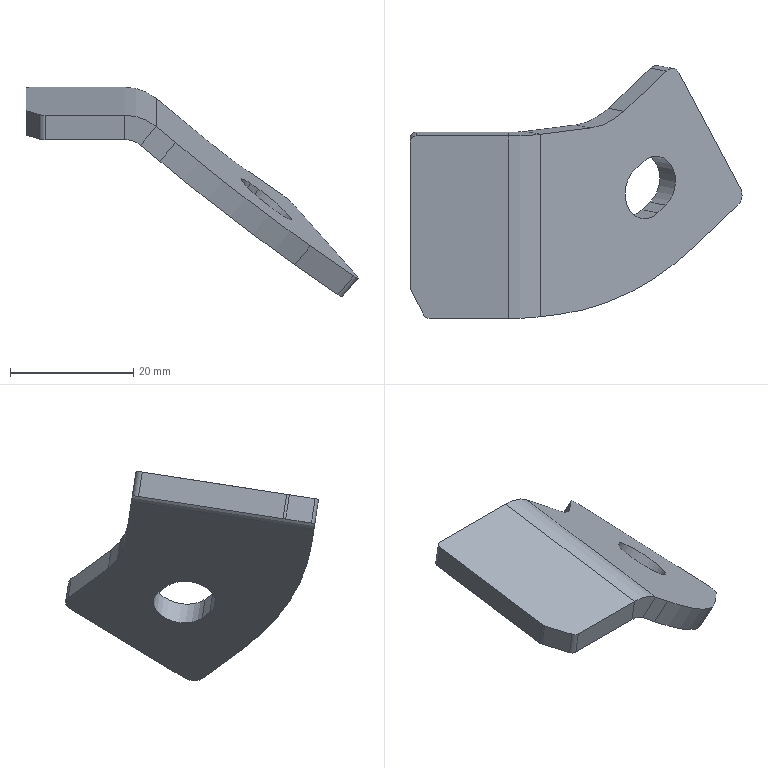Part | SolidWorks | features BaseBody 1 | 1 solid | 28 faces | box 53.982 x 41.139 x 34.078 mm | volume 6539 mm3 | plane 16 | cylinder 11 | spline 1 | commonest cylinder face diameters 2 x3 4 x2 9 x2 8 x1 16 x1 26 x1
STEP:
#1=CARTESIAN_POINT('',(-301.692,285.702,-816.532));
#2=VERTEX_POINT('',#1);
#3=CARTESIAN_POINT('',(-299.57,281.523,-817.174));
#4=VERTEX_POINT('',#3);
#5=CARTESIAN_POINT('',(-301.692,285.702,-816.532));
#6=CARTESIAN_POINT('',(-301.439,285.211,-816.607));
#7=CARTESIAN_POINT('',(-300.904,284.166,-816.768));
#8=CARTESIAN_POINT('',(-300.195,282.773,-816.982));
#9=CARTESIAN_POINT('',(-299.746,281.876,-817.12));
#10=CARTESIAN_POINT('',(-299.57,281.523,-817.174));
#11=B_SPLINE_CURVE_WITH_KNOTS('',3,(#5,#6,#7,#8,#9,#10),.UNSPECIFIED.,.F.,.F.,(4,1,1,4),(0.,0.3455,0.7405,1.),.UNSPECIFIED.);
#12=EDGE_CURVE('',#2,#4,#11,.T.);
#13=ORIENTED_EDGE('',*,*,#12,.F.);
#14=CARTESIAN_POINT('',(-301.8,286.15,-816.463));
#15=VERTEX_POINT('',#14);
#16=CARTESIAN_POINT('',(-300.8,286.15,-816.463));
#17=DIRECTION('',(0.,-0.1519,0.9884));
#18=DIRECTION('',(-1.,0.,0.));
#19=AXIS2_PLACEMENT_3D('',#16,#17,#18);
#20=CIRCLE('',#19,1.);
#21=EDGE_CURVE('',#15,#2,#20,.T.);
#22=ORIENTED_EDGE('',*,*,#21,.F.);
#23=CARTESIAN_POINT('',(-301.8,309.634,-812.853));
#24=VERTEX_POINT('',#23);
#25=CARTESIAN_POINT('',(-301.8,286.15,-816.463));
#26=DIRECTION('',(0.,0.9884,0.1519));
#27=VECTOR('',#26,1000.);
#28=LINE('',#25,#27);
#29=EDGE_CURVE('',#15,#24,#28,.T.);
#30=ORIENTED_EDGE('',*,*,#29,.T.);
#31=CARTESIAN_POINT('',(-300.8,310.623,-812.701));
#32=VERTEX_POINT('',#31);
#33=CARTESIAN_POINT('',(-300.8,309.634,-812.853));
#34=DIRECTION('',(0.,-0.1519,0.9884));
#35=DIRECTION('',(0.,0.9884,0.1519));
#36=AXIS2_PLACEMENT_3D('',#33,#34,#35);
#37=CIRCLE('',#36,1.);
#38=EDGE_CURVE('',#32,#24,#37,.T.);
#39=ORIENTED_EDGE('',*,*,#38,.F.);
#40=CARTESIAN_POINT('',(-285.757,310.623,-812.701));
#41=VERTEX_POINT('',#40);
#42=CARTESIAN_POINT('',(-300.8,310.623,-812.701));
#43=DIRECTION('',(1.,0.,0.));
#44=VECTOR('',#43,1000.);
#45=LINE('',#42,#44);
#46=EDGE_CURVE('',#32,#41,#45,.T.);
#47=ORIENTED_EDGE('',*,*,#46,.T.);
#48=CARTESIAN_POINT('',(-285.757,280.971,-817.259));
#49=VERTEX_POINT('',#48);
#50=CARTESIAN_POINT('',(-285.757,310.623,-812.701));
#51=DIRECTION('',(0.,-0.9884,-0.1519));
#52=VECTOR('',#51,1000.);
#53=LINE('',#50,#52);
#54=EDGE_CURVE('',#41,#49,#53,.T.);
#55=ORIENTED_EDGE('',*,*,#54,.T.);
#56=CARTESIAN_POINT('',(-298.673,280.971,-817.259));
#57=VERTEX_POINT('',#56);
#58=CARTESIAN_POINT('',(-285.757,280.971,-817.259));
#59=DIRECTION('',(-1.,0.,0.));
#60=VECTOR('',#59,1000.);
#61=LINE('',#58,#60);
#62=EDGE_CURVE('',#49,#57,#61,.T.);
#63=ORIENTED_EDGE('',*,*,#62,.T.);
#64=CARTESIAN_POINT('',(-298.673,281.959,-817.107));
#65=DIRECTION('',(0.,-0.1519,0.9884));
#66=DIRECTION('',(-0.8972,-0.4365,-0.0671));
#67=AXIS2_PLACEMENT_3D('',#64,#65,#66);
#68=CIRCLE('',#67,1.);
#69=EDGE_CURVE('',#4,#57,#68,.T.);
#70=ORIENTED_EDGE('',*,*,#69,.F.);
#71=EDGE_LOOP('',(#13,#22,#30,#39,#47,#55,#63,#70));
#72=FACE_OUTER_BOUND('',#71,.T.);
#73=CARTESIAN_POINT('',(-79.9,310.623,-812.701));
#74=DIRECTION('',(0.,-0.1519,0.9884));
#75=DIRECTION('',(-1.,0.,0.));
#76=AXIS2_PLACEMENT_3D('',#73,#74,#75);
#77=PLANE('',#76);
#78=ADVANCED_FACE('',(#72),#77,.F.);
#79=CARTESIAN_POINT('',(-298.673,280.363,-813.306));
#80=VERTEX_POINT('',#79);
#81=CARTESIAN_POINT('',(-298.673,280.363,-813.306));
#82=DIRECTION('',(0.,0.1519,-0.9884));
#83=VECTOR('',#82,1000.);
#84=LINE('',#81,#83);
#85=EDGE_CURVE('',#80,#57,#84,.T.);
#86=ORIENTED_EDGE('',*,*,#85,.F.);
#87=CARTESIAN_POINT('',(-299.57,280.915,-813.221));
#88=VERTEX_POINT('',#87);
#89=CARTESIAN_POINT('',(-298.673,281.352,-813.154));
#90=DIRECTION('',(0.,0.1519,-0.9884));
#91=DIRECTION('',(0.,-0.9884,-0.1519));
#92=AXIS2_PLACEMENT_3D('',#89,#90,#91);
#93=CIRCLE('',#92,1.);
#94=EDGE_CURVE('',#80,#88,#93,.T.);
#95=ORIENTED_EDGE('',*,*,#94,.T.);
#96=CARTESIAN_POINT('',(-299.57,281.523,-817.174));
#97=DIRECTION('',(0.,-0.1519,0.9884));
#98=VECTOR('',#97,1000.);
#99=LINE('',#96,#98);
#100=EDGE_CURVE('',#4,#88,#99,.T.);
#101=ORIENTED_EDGE('',*,*,#100,.F.);
#102=ORIENTED_EDGE('',*,*,#69,.T.);
#103=EDGE_LOOP('',(#86,#95,#101,#102));
#104=FACE_OUTER_BOUND('',#103,.T.);
#105=CARTESIAN_POINT('',(-298.673,281.656,-815.131));
#106=DIRECTION('',(0.,0.1519,-0.9884));
#107=DIRECTION('',(0.,-0.9884,-0.1519));
#108=AXIS2_PLACEMENT_3D('',#105,#106,#107);
#109=CYLINDRICAL_SURFACE('',#108,1.);
#110=ADVANCED_FACE('',(#104),#109,.T.);
#111=CARTESIAN_POINT('',(-301.692,285.094,-812.578));
#112=VERTEX_POINT('',#111);
#113=CARTESIAN_POINT('',(-299.57,280.915,-813.221));
#114=CARTESIAN_POINT('',(-299.746,281.269,-813.166));
#115=CARTESIAN_POINT('',(-300.195,282.166,-813.029));
#116=CARTESIAN_POINT('',(-300.904,283.558,-812.815));
#117=CARTESIAN_POINT('',(-301.439,284.603,-812.654));
#118=CARTESIAN_POINT('',(-301.692,285.094,-812.578));
#119=B_SPLINE_CURVE_WITH_KNOTS('',3,(#113,#114,#115,#116,#117,#118),.UNSPECIFIED.,.F.,.F.,(4,1,1,4),(0.,0.2595,0.6545,1.),.UNSPECIFIED.);
#120=EDGE_CURVE('',#88,#112,#119,.T.);
#121=ORIENTED_EDGE('',*,*,#120,.T.);
#122=CARTESIAN_POINT('',(-301.692,285.094,-812.578));
#123=DIRECTION('',(0.,0.1519,-0.9884));
#124=VECTOR('',#123,1000.);
#125=LINE('',#122,#124);
#126=EDGE_CURVE('',#112,#2,#125,.T.);
#127=ORIENTED_EDGE('',*,*,#126,.T.);
#128=ORIENTED_EDGE('',*,*,#12,.T.);
#129=ORIENTED_EDGE('',*,*,#100,.T.);
#130=EDGE_LOOP('',(#121,#127,#128,#129));
#131=FACE_OUTER_BOUND('',#130,.T.);
#132=CARTESIAN_POINT('',(-301.692,285.702,-816.532));
#133=CARTESIAN_POINT('',(-301.692,285.094,-812.578));
#134=CARTESIAN_POINT('',(-301.439,285.211,-816.607));
#135=CARTESIAN_POINT('',(-301.439,284.603,-812.654));
#136=CARTESIAN_POINT('',(-300.904,284.166,-816.768));
#137=CARTESIAN_POINT('',(-300.904,283.558,-812.815));
#138=CARTESIAN_POINT('',(-300.195,282.773,-816.982));
#139=CARTESIAN_POINT('',(-300.195,282.166,-813.029));
#140=CARTESIAN_POINT('',(-299.746,281.876,-817.12));
#141=CARTESIAN_POINT('',(-299.746,281.269,-813.166));
#142=CARTESIAN_POINT('',(-299.57,281.523,-817.174));
#143=CARTESIAN_POINT('',(-299.57,280.915,-813.221));
#144=B_SPLINE_SURFACE_WITH_KNOTS('',3,1,((#132,#133),(#134,#135),(#136,#137),(#138,#139),(#140,#141),(#142,#143)),.UNSPECIFIED.,.F.,.F.,.F.,(4,1,1,4),(2,2),(0.0124,0.3492,0.7341,0.987),(0.,1.),.UNSPECIFIED.);
#145=ADVANCED_FACE('',(#131),#144,.T.);
#146=CARTESIAN_POINT('',(-301.8,285.542,-812.51));
#147=VERTEX_POINT('',#146);
#148=CARTESIAN_POINT('',(-301.8,286.15,-816.463));
#149=DIRECTION('',(0.,-0.1519,0.9884));
#150=VECTOR('',#149,1000.);
#151=LINE('',#148,#150);
#152=EDGE_CURVE('',#15,#147,#151,.T.);
#153=ORIENTED_EDGE('',*,*,#152,.F.);
#154=ORIENTED_EDGE('',*,*,#21,.T.);
#155=ORIENTED_EDGE('',*,*,#126,.F.);
#156=CARTESIAN_POINT('',(-300.8,285.542,-812.51));
#157=DIRECTION('',(0.,0.1519,-0.9884));
#158=DIRECTION('',(-0.8916,-0.4476,-0.0688));
#159=AXIS2_PLACEMENT_3D('',#156,#157,#158);
#160=CIRCLE('',#159,1.);
#161=EDGE_CURVE('',#112,#147,#160,.T.);
#162=ORIENTED_EDGE('',*,*,#161,.T.);
#163=EDGE_LOOP('',(#153,#154,#155,#162));
#164=FACE_OUTER_BOUND('',#163,.T.);
#165=CARTESIAN_POINT('',(-300.8,285.846,-814.486));
#166=DIRECTION('',(0.,-0.1519,0.9884));
#167=DIRECTION('',(-1.,0.,0.));
#168=AXIS2_PLACEMENT_3D('',#165,#166,#167);
#169=CYLINDRICAL_SURFACE('',#168,1.);
#170=ADVANCED_FACE('',(#164),#169,.T.);
#171=CARTESIAN_POINT('',(-285.757,280.363,-813.306));
#172=VERTEX_POINT('',#171);
#173=CARTESIAN_POINT('',(-285.757,280.363,-813.306));
#174=DIRECTION('',(-1.,0.,0.));
#175=VECTOR('',#174,1000.);
#176=LINE('',#173,#175);
#177=EDGE_CURVE('',#172,#80,#176,.T.);
#178=ORIENTED_EDGE('',*,*,#177,.F.);
#179=CARTESIAN_POINT('',(-285.757,310.015,-808.748));
#180=VERTEX_POINT('',#179);
#181=CARTESIAN_POINT('',(-285.757,280.363,-813.306));
#182=DIRECTION('',(0.,0.9884,0.1519));
#183=VECTOR('',#182,1000.);
#184=LINE('',#181,#183);
#185=EDGE_CURVE('',#172,#180,#184,.T.);
#186=ORIENTED_EDGE('',*,*,#185,.T.);
#187=CARTESIAN_POINT('',(-300.8,310.015,-808.748));
#188=VERTEX_POINT('',#187);
#189=CARTESIAN_POINT('',(-300.8,310.015,-808.748));
#190=DIRECTION('',(1.,0.,0.));
#191=VECTOR('',#190,1000.);
#192=LINE('',#189,#191);
#193=EDGE_CURVE('',#188,#180,#192,.T.);
#194=ORIENTED_EDGE('',*,*,#193,.F.);
#195=CARTESIAN_POINT('',(-301.8,309.027,-808.9));
#196=VERTEX_POINT('',#195);
#197=CARTESIAN_POINT('',(-300.8,309.027,-808.9));
#198=DIRECTION('',(0.,0.1519,-0.9884));
#199=DIRECTION('',(-1.,0.,0.));
#200=AXIS2_PLACEMENT_3D('',#197,#198,#199);
#201=CIRCLE('',#200,1.);
#202=EDGE_CURVE('',#196,#188,#201,.T.);
#203=ORIENTED_EDGE('',*,*,#202,.F.);
#204=CARTESIAN_POINT('',(-301.8,285.542,-812.51));
#205=DIRECTION('',(0.,0.9884,0.1519));
#206=VECTOR('',#205,1000.);
#207=LINE('',#204,#206);
#208=EDGE_CURVE('',#147,#196,#207,.T.);
#209=ORIENTED_EDGE('',*,*,#208,.F.);
#210=ORIENTED_EDGE('',*,*,#161,.F.);
#211=ORIENTED_EDGE('',*,*,#120,.F.);
#212=ORIENTED_EDGE('',*,*,#94,.F.);
#213=EDGE_LOOP('',(#178,#186,#194,#203,#209,#210,#211,#212));
#214=FACE_OUTER_BOUND('',#213,.T.);
#215=CARTESIAN_POINT('',(-79.9,310.015,-808.748));
#216=DIRECTION('',(0.,-0.1519,0.9884));
#217=DIRECTION('',(-1.,0.,0.));
#218=AXIS2_PLACEMENT_3D('',#215,#216,#217);
#219=PLANE('',#218);
#220=ADVANCED_FACE('',(#214),#219,.T.);
#221=ORIENTED_EDGE('',*,*,#208,.T.);
#222=CARTESIAN_POINT('',(-301.8,309.027,-808.9));
#223=DIRECTION('',(0.,0.1519,-0.9884));
#224=VECTOR('',#223,1000.);
#225=LINE('',#222,#224);
#226=EDGE_CURVE('',#196,#24,#225,.T.);
#227=ORIENTED_EDGE('',*,*,#226,.T.);
#228=ORIENTED_EDGE('',*,*,#29,.F.);
#229=ORIENTED_EDGE('',*,*,#152,.T.);
#230=EDGE_LOOP('',(#221,#227,#228,#229));
#231=FACE_OUTER_BOUND('',#230,.T.);
#232=CARTESIAN_POINT('',(-301.8,310.015,-808.748));
#233=DIRECTION('',(-1.,0.,0.));
#234=DIRECTION('',(0.,0.,1.));
#235=AXIS2_PLACEMENT_3D('',#232,#233,#234);
#236=PLANE('',#235);
#237=ADVANCED_FACE('',(#231),#236,.T.);
#238=ORIENTED_EDGE('',*,*,#226,.F.);
#239=ORIENTED_EDGE('',*,*,#202,.T.);
#240=CARTESIAN_POINT('',(-300.8,310.623,-812.701));
#241=DIRECTION('',(0.,-0.1519,0.9884));
#242=VECTOR('',#241,1000.);
#243=LINE('',#240,#242);
#244=EDGE_CURVE('',#32,#188,#243,.T.);
#245=ORIENTED_EDGE('',*,*,#244,.F.);
#246=ORIENTED_EDGE('',*,*,#38,.T.);
#247=EDGE_LOOP('',(#238,#239,#245,#246));
#248=FACE_OUTER_BOUND('',#247,.T.);
#249=CARTESIAN_POINT('',(-300.8,286.049,-659.424));
#250=DIRECTION('',(0.,-0.1519,0.9884));
#251=DIRECTION('',(0.,0.9884,0.1519));
#252=AXIS2_PLACEMENT_3D('',#249,#250,#251);
#253=CYLINDRICAL_SURFACE('',#252,1.);
#254=ADVANCED_FACE('',(#248),#253,.T.);
#255=ORIENTED_EDGE('',*,*,#193,.T.);
#256=CARTESIAN_POINT('',(-285.757,310.015,-808.748));
#257=DIRECTION('',(0.,0.1519,-0.9884));
#258=VECTOR('',#257,1000.);
#259=LINE('',#256,#258);
#260=EDGE_CURVE('',#180,#41,#259,.T.);
#261=ORIENTED_EDGE('',*,*,#260,.T.);
#262=ORIENTED_EDGE('',*,*,#46,.F.);
#263=ORIENTED_EDGE('',*,*,#244,.T.);
#264=EDGE_LOOP('',(#255,#261,#262,#263));
#265=FACE_OUTER_BOUND('',#264,.T.);
#266=CARTESIAN_POINT('',(-296.192,310.319,-810.724));
#267=DIRECTION('',(0.,-0.9884,-0.1519));
#268=DIRECTION('',(0.,0.1519,-0.9884));
#269=AXIS2_PLACEMENT_3D('',#266,#267,#268);
#270=PLANE('',#269);
#271=ADVANCED_FACE('',(#265),#270,.F.);
#272=ORIENTED_EDGE('',*,*,#260,.F.);
#273=CARTESIAN_POINT('',(-280.635,310.297,-810.581));
#274=VERTEX_POINT('',#273);
#275=CARTESIAN_POINT('',(-285.757,311.23,-816.655));
#276=DIRECTION('',(0.,-0.9884,-0.1519));
#277=DIRECTION('',(0.6403,-0.1167,0.7592));
#278=AXIS2_PLACEMENT_3D('',#275,#276,#277);
#279=CIRCLE('',#278,8.);
#280=EDGE_CURVE('',#274,#180,#279,.T.);
#281=ORIENTED_EDGE('',*,*,#280,.F.);
#282=CARTESIAN_POINT('',(-283.196,310.764,-813.618));
#283=VERTEX_POINT('',#282);
#284=CARTESIAN_POINT('',(-283.196,310.764,-813.618));
#285=DIRECTION('',(0.6403,-0.1167,0.7592));
#286=VECTOR('',#285,1000.);
#287=LINE('',#284,#286);
#288=EDGE_CURVE('',#283,#274,#287,.T.);
#289=ORIENTED_EDGE('',*,*,#288,.F.);
#290=CARTESIAN_POINT('',(-285.757,311.23,-816.655));
#291=DIRECTION('',(0.,0.9884,0.1519));
#292=DIRECTION('',(0.,-0.1519,0.9884));
#293=AXIS2_PLACEMENT_3D('',#290,#291,#292);
#294=CIRCLE('',#293,4.);
#295=EDGE_CURVE('',#41,#283,#294,.T.);
#296=ORIENTED_EDGE('',*,*,#295,.F.);
#297=EDGE_LOOP('',(#272,#281,#289,#296));
#298=FACE_OUTER_BOUND('',#297,.T.);
#299=CARTESIAN_POINT('',(-283.715,310.373,-811.079));
#300=DIRECTION('',(0.,0.9884,0.1519));
#301=DIRECTION('',(1.,0.,0.));
#302=AXIS2_PLACEMENT_3D('',#299,#300,#301);
#303=PLANE('',#302);
#304=ADVANCED_FACE('',(#298),#303,.T.);
#305=ORIENTED_EDGE('',*,*,#295,.T.);
#306=CARTESIAN_POINT('',(-283.196,281.112,-818.176));
#307=VERTEX_POINT('',#306);
#308=CARTESIAN_POINT('',(-283.196,281.112,-818.176));
#309=DIRECTION('',(0.,0.9884,0.1519));
#310=VECTOR('',#309,1000.);
#311=LINE('',#308,#310);
#312=EDGE_CURVE('',#307,#283,#311,.T.);
#313=ORIENTED_EDGE('',*,*,#312,.F.);
#314=CARTESIAN_POINT('',(-285.757,281.579,-821.213));
#315=DIRECTION('',(0.,-0.9884,-0.1519));
#316=DIRECTION('',(0.6403,-0.1167,0.7592));
#317=AXIS2_PLACEMENT_3D('',#314,#315,#316);
#318=CIRCLE('',#317,4.);
#319=EDGE_CURVE('',#307,#49,#318,.T.);
#320=ORIENTED_EDGE('',*,*,#319,.T.);
#321=ORIENTED_EDGE('',*,*,#54,.F.);
#322=EDGE_LOOP('',(#305,#313,#320,#321));
#323=FACE_OUTER_BOUND('',#322,.T.);
#324=CARTESIAN_POINT('',(-285.757,457.66,-794.146));
#325=DIRECTION('',(0.,0.9884,0.1519));
#326=DIRECTION('',(0.,-0.1519,0.9884));
#327=AXIS2_PLACEMENT_3D('',#324,#325,#326);
#328=CYLINDRICAL_SURFACE('',#327,4.);
#329=ADVANCED_FACE('',(#323),#328,.F.);
#330=CARTESIAN_POINT('',(-280.635,280.645,-815.139));
#331=VERTEX_POINT('',#330);
#332=CARTESIAN_POINT('',(-280.635,280.645,-815.139));
#333=DIRECTION('',(-0.6403,0.1167,-0.7592));
#334=VECTOR('',#333,1000.);
#335=LINE('',#332,#334);
#336=EDGE_CURVE('',#331,#307,#335,.T.);
#337=ORIENTED_EDGE('',*,*,#336,.F.);
#338=CARTESIAN_POINT('',(-285.757,281.579,-821.213));
#339=DIRECTION('',(0.,0.9884,0.1519));
#340=DIRECTION('',(0.,-0.1519,0.9884));
#341=AXIS2_PLACEMENT_3D('',#338,#339,#340);
#342=CIRCLE('',#341,8.);
#343=EDGE_CURVE('',#172,#331,#342,.T.);
#344=ORIENTED_EDGE('',*,*,#343,.F.);
#345=CARTESIAN_POINT('',(-285.757,280.971,-817.259));
#346=DIRECTION('',(0.,-0.1519,0.9884));
#347=VECTOR('',#346,1000.);
#348=LINE('',#345,#347);
#349=EDGE_CURVE('',#49,#172,#348,.T.);
#350=ORIENTED_EDGE('',*,*,#349,.F.);
#351=ORIENTED_EDGE('',*,*,#319,.F.);
#352=EDGE_LOOP('',(#337,#344,#350,#351));
#353=FACE_OUTER_BOUND('',#352,.T.);
#354=CARTESIAN_POINT('',(-283.715,280.722,-815.637));
#355=DIRECTION('',(0.,-0.9884,-0.1519));
#356=DIRECTION('',(0.,0.1519,-0.9884));
#357=AXIS2_PLACEMENT_3D('',#354,#355,#356);
#358=PLANE('',#357);
#359=ADVANCED_FACE('',(#353),#358,.T.);
#360=ORIENTED_EDGE('',*,*,#62,.F.);
#361=ORIENTED_EDGE('',*,*,#349,.T.);
#362=ORIENTED_EDGE('',*,*,#177,.T.);
#363=ORIENTED_EDGE('',*,*,#85,.T.);
#364=EDGE_LOOP('',(#360,#361,#362,#363));
#365=FACE_OUTER_BOUND('',#364,.T.);
#366=CARTESIAN_POINT('',(-292.527,280.667,-815.282));
#367=DIRECTION('',(0.,0.9884,0.1519));
#368=DIRECTION('',(1.,0.,0.));
#369=AXIS2_PLACEMENT_3D('',#366,#367,#368);
#370=PLANE('',#369);
#371=ADVANCED_FACE('',(#365),#370,.F.);
#372=ORIENTED_EDGE('',*,*,#343,.T.);
#373=CARTESIAN_POINT('',(-280.635,310.297,-810.581));
#374=DIRECTION('',(0.,-0.9884,-0.1519));
#375=VECTOR('',#374,1000.);
#376=LINE('',#373,#375);
#377=EDGE_CURVE('',#274,#331,#376,.T.);
#378=ORIENTED_EDGE('',*,*,#377,.F.);
#379=ORIENTED_EDGE('',*,*,#280,.T.);
#380=ORIENTED_EDGE('',*,*,#185,.F.);
#381=EDGE_LOOP('',(#372,#378,#379,#380));
#382=FACE_OUTER_BOUND('',#381,.T.);
#383=CARTESIAN_POINT('',(-285.757,457.66,-794.146));
#384=DIRECTION('',(0.,0.9884,0.1519));
#385=DIRECTION('',(0.,-0.1519,0.9884));
#386=AXIS2_PLACEMENT_3D('',#383,#384,#385);
#387=CYLINDRICAL_SURFACE('',#386,8.);
#388=ADVANCED_FACE('',(#382),#387,.T.);
#389=CARTESIAN_POINT('',(-263.963,305.811,-825.33));
#390=VERTEX_POINT('',#389);
#391=CARTESIAN_POINT('',(-265.255,304.579,-824.429));
#392=VERTEX_POINT('',#391);
#393=CARTESIAN_POINT('',(-263.963,305.811,-825.33));
#394=DIRECTION('',(-0.6461,-0.6164,0.4501));
#395=VECTOR('',#394,1000.);
#396=LINE('',#393,#395);
#397=EDGE_CURVE('',#390,#392,#396,.T.);
#398=ORIENTED_EDGE('',*,*,#397,.F.);
#399=CARTESIAN_POINT('',(-260.224,298.803,-829.56));
#400=VERTEX_POINT('',#399);
#401=CARTESIAN_POINT('',(-262.093,302.307,-827.445));
#402=DIRECTION('',(0.6403,-0.1167,0.7592));
#403=DIRECTION('',(0.4155,-0.7787,-0.4701));
#404=AXIS2_PLACEMENT_3D('',#401,#402,#403);
#405=CIRCLE('',#404,4.5);
#406=EDGE_CURVE('',#400,#390,#405,.T.);
#407=ORIENTED_EDGE('',*,*,#406,.F.);
#408=CARTESIAN_POINT('',(-261.516,297.57,-828.66));
#409=VERTEX_POINT('',#408);
#410=CARTESIAN_POINT('',(-261.516,297.57,-828.66));
#411=DIRECTION('',(0.6461,0.6164,-0.4501));
#412=VECTOR('',#411,1000.);
#413=LINE('',#410,#412);
#414=EDGE_CURVE('',#409,#400,#413,.T.);
#415=ORIENTED_EDGE('',*,*,#414,.F.);
#416=CARTESIAN_POINT('',(-263.386,301.074,-826.545));
#417=DIRECTION('',(0.6403,-0.1167,0.7592));
#418=DIRECTION('',(-0.4155,0.7787,0.4701));
#419=AXIS2_PLACEMENT_3D('',#416,#417,#418);
#420=CIRCLE('',#419,4.5);
#421=EDGE_CURVE('',#392,#409,#420,.T.);
#422=ORIENTED_EDGE('',*,*,#421,.F.);
#423=EDGE_LOOP('',(#398,#407,#415,#422));
#424=FACE_BOUND('',#423,.T.);
#425=CARTESIAN_POINT('',(-248.523,298.802,-839.427));
#426=VERTEX_POINT('',#425);
#427=CARTESIAN_POINT('',(-255.53,292.117,-834.546));
#428=VERTEX_POINT('',#427);
#429=CARTESIAN_POINT('',(-248.523,298.802,-839.427));
#430=DIRECTION('',(-0.6461,-0.6164,0.4501));
#431=VECTOR('',#430,1000.);
#432=LINE('',#429,#431);
#433=EDGE_CURVE('',#426,#428,#432,.T.);
#434=ORIENTED_EDGE('',*,*,#433,.F.);
#435=CARTESIAN_POINT('',(-248.062,301.593,-839.387));
#436=VERTEX_POINT('',#435);
#437=CARTESIAN_POINT('',(-249.354,300.36,-838.487));
#438=DIRECTION('',(-0.6403,0.1167,-0.7592));
#439=DIRECTION('',(0.6461,0.6164,-0.4501));
#440=AXIS2_PLACEMENT_3D('',#437,#438,#439);
#441=CIRCLE('',#440,2.);
#442=EDGE_CURVE('',#436,#426,#441,.T.);
#443=ORIENTED_EDGE('',*,*,#442,.F.);
#444=CARTESIAN_POINT('',(-258.034,320.282,-828.105));
#445=VERTEX_POINT('',#444);
#446=CARTESIAN_POINT('',(-258.034,320.282,-828.105));
#447=DIRECTION('',(0.4155,-0.7787,-0.4701));
#448=VECTOR('',#447,1000.);
#449=LINE('',#446,#448);
#450=EDGE_CURVE('',#445,#436,#449,.T.);
#451=ORIENTED_EDGE('',*,*,#450,.F.);
#452=CARTESIAN_POINT('',(-260.157,320.606,-826.265));
#453=VERTEX_POINT('',#452);
#454=CARTESIAN_POINT('',(-259.326,319.049,-827.205));
#455=DIRECTION('',(-0.6403,0.1167,-0.7592));
#456=DIRECTION('',(-0.4155,0.7787,0.4701));
#457=AXIS2_PLACEMENT_3D('',#454,#455,#456);
#458=CIRCLE('',#457,2.);
#459=EDGE_CURVE('',#453,#445,#458,.T.);
#460=ORIENTED_EDGE('',*,*,#459,.F.);
#461=CARTESIAN_POINT('',(-267.015,314.063,-821.488));
#462=VERTEX_POINT('',#461);
#463=CARTESIAN_POINT('',(-267.015,314.063,-821.488));
#464=DIRECTION('',(0.6461,0.6164,-0.4501));
#465=VECTOR('',#464,1000.);
#466=LINE('',#463,#465);
#467=EDGE_CURVE('',#462,#453,#466,.T.);
#468=ORIENTED_EDGE('',*,*,#467,.F.);
#469=CARTESIAN_POINT('',(-272.416,311.338,-817.352));
#470=VERTEX_POINT('',#469);
#471=CARTESIAN_POINT('',(-272.416,324.187,-815.377));
#472=DIRECTION('',(0.6403,-0.1167,0.7592));
#473=DIRECTION('',(0.,-0.9884,-0.1519));
#474=AXIS2_PLACEMENT_3D('',#471,#472,#473);
#475=CIRCLE('',#474,13.);
#476=EDGE_CURVE('',#470,#462,#475,.T.);
#477=ORIENTED_EDGE('',*,*,#476,.F.);
#478=CARTESIAN_POINT('',(-272.416,311.338,-817.352));
#479=DIRECTION('',(-0.7682,-0.09728,0.6328));
#480=VECTOR('',#479,1000.);
#481=LINE('',#478,#480);
#482=EDGE_CURVE('',#470,#274,#481,.T.);
#483=ORIENTED_EDGE('',*,*,#482,.T.);
#484=ORIENTED_EDGE('',*,*,#377,.T.);
#485=CARTESIAN_POINT('',(-277.468,281.046,-817.748));
#486=VERTEX_POINT('',#485);
#487=CARTESIAN_POINT('',(-280.635,280.645,-815.139));
#488=DIRECTION('',(0.7682,0.09728,-0.6328));
#489=VECTOR('',#488,1000.);
#490=LINE('',#487,#489);
#491=EDGE_CURVE('',#331,#486,#490,.T.);
#492=ORIENTED_EDGE('',*,*,#491,.T.);
#493=CARTESIAN_POINT('',(-277.468,333.233,-809.726));
#494=DIRECTION('',(-0.6403,0.1167,-0.7592));
#495=DIRECTION('',(0.4155,-0.7787,-0.4701));
#496=AXIS2_PLACEMENT_3D('',#493,#494,#495);
#497=CIRCLE('',#496,52.8);
#498=EDGE_CURVE('',#428,#486,#497,.T.);
#499=ORIENTED_EDGE('',*,*,#498,.F.);
#500=EDGE_LOOP('',(#434,#443,#451,#460,#468,#477,#483,#484,#492,#499));
#501=FACE_OUTER_BOUND('',#500,.T.);
#502=CARTESIAN_POINT('',(-579.404,91.053,-592.338));
#503=DIRECTION('',(-0.6403,0.1167,-0.7592));
#504=DIRECTION('',(-0.7645,0.,0.6447));
#505=AXIS2_PLACEMENT_3D('',#502,#503,#504);
#506=PLANE('',#505);
#507=ADVANCED_FACE('',(#424,#501),#506,.F.);
#508=CARTESIAN_POINT('',(-258.091,292.584,-837.583));
#509=VERTEX_POINT('',#508);
#510=CARTESIAN_POINT('',(-255.53,292.117,-834.546));
#511=DIRECTION('',(-0.6403,0.1167,-0.7592));
#512=VECTOR('',#511,1000.);
#513=LINE('',#510,#512);
#514=EDGE_CURVE('',#428,#509,#513,.T.);
#515=ORIENTED_EDGE('',*,*,#514,.F.);
#516=ORIENTED_EDGE('',*,*,#498,.T.);
#517=CARTESIAN_POINT('',(-280.029,281.513,-820.785));
#518=VERTEX_POINT('',#517);
#519=CARTESIAN_POINT('',(-280.029,281.513,-820.785));
#520=DIRECTION('',(0.6403,-0.1167,0.7592));
#521=VECTOR('',#520,1000.);
#522=LINE('',#519,#521);
#523=EDGE_CURVE('',#518,#486,#522,.T.);
#524=ORIENTED_EDGE('',*,*,#523,.F.);
#525=CARTESIAN_POINT('',(-280.029,333.7,-812.763));
#526=DIRECTION('',(0.6403,-0.1167,0.7592));
#527=DIRECTION('',(0.,-0.9884,-0.1519));
#528=AXIS2_PLACEMENT_3D('',#525,#526,#527);
#529=CIRCLE('',#528,52.8);
#530=EDGE_CURVE('',#518,#509,#529,.T.);
#531=ORIENTED_EDGE('',*,*,#530,.T.);
#532=EDGE_LOOP('',(#515,#516,#524,#531));
#533=FACE_OUTER_BOUND('',#532,.T.);
#534=CARTESIAN_POINT('',(-196.23,318.424,-713.389));
#535=DIRECTION('',(0.6403,-0.1167,0.7592));
#536=DIRECTION('',(0.,-0.9884,-0.1519));
#537=AXIS2_PLACEMENT_3D('',#534,#535,#536);
#538=CYLINDRICAL_SURFACE('',#537,52.8);
#539=ADVANCED_FACE('',(#533),#538,.T.);
#540=CARTESIAN_POINT('',(-262.785,299.27,-832.597));
#541=VERTEX_POINT('',#540);
#542=CARTESIAN_POINT('',(-264.077,298.037,-831.697));
#543=VERTEX_POINT('',#542);
#544=CARTESIAN_POINT('',(-262.785,299.27,-832.597));
#545=DIRECTION('',(-0.6461,-0.6164,0.4501));
#546=VECTOR('',#545,1000.);
#547=LINE('',#544,#546);
#548=EDGE_CURVE('',#541,#543,#547,.T.);
#549=ORIENTED_EDGE('',*,*,#548,.F.);
#550=CARTESIAN_POINT('',(-266.524,306.278,-828.367));
#551=VERTEX_POINT('',#550);
#552=CARTESIAN_POINT('',(-264.654,302.774,-830.482));
#553=DIRECTION('',(-0.6403,0.1167,-0.7592));
#554=DIRECTION('',(-0.4155,0.7787,0.4701));
#555=AXIS2_PLACEMENT_3D('',#552,#553,#554);
#556=CIRCLE('',#555,4.5);
#557=EDGE_CURVE('',#551,#541,#556,.T.);
#558=ORIENTED_EDGE('',*,*,#557,.F.);
#559=CARTESIAN_POINT('',(-267.816,305.045,-827.466));
#560=VERTEX_POINT('',#559);
#561=CARTESIAN_POINT('',(-267.816,305.045,-827.466));
#562=DIRECTION('',(0.6461,0.6164,-0.4501));
#563=VECTOR('',#562,1000.);
#564=LINE('',#561,#563);
#565=EDGE_CURVE('',#560,#551,#564,.T.);
#566=ORIENTED_EDGE('',*,*,#565,.F.);
#567=CARTESIAN_POINT('',(-265.947,301.541,-829.582));
#568=DIRECTION('',(-0.6403,0.1167,-0.7592));
#569=DIRECTION('',(0.4155,-0.7787,-0.4701));
#570=AXIS2_PLACEMENT_3D('',#567,#568,#569);
#571=CIRCLE('',#570,4.5);
#572=EDGE_CURVE('',#543,#560,#571,.T.);
#573=ORIENTED_EDGE('',*,*,#572,.F.);
#574=EDGE_LOOP('',(#549,#558,#566,#573));
#575=FACE_BOUND('',#574,.T.);
#576=CARTESIAN_POINT('',(-283.196,281.112,-818.176));
#577=DIRECTION('',(0.7682,0.09728,-0.6328));
#578=VECTOR('',#577,1000.);
#579=LINE('',#576,#578);
#580=EDGE_CURVE('',#307,#518,#579,.T.);
#581=ORIENTED_EDGE('',*,*,#580,.F.);
#582=ORIENTED_EDGE('',*,*,#312,.T.);
#583=CARTESIAN_POINT('',(-274.977,311.804,-820.389));
#584=VERTEX_POINT('',#583);
#585=CARTESIAN_POINT('',(-274.977,311.804,-820.389));
#586=DIRECTION('',(-0.7682,-0.09728,0.6328));
#587=VECTOR('',#586,1000.);
#588=LINE('',#585,#587);
#589=EDGE_CURVE('',#584,#283,#588,.T.);
#590=ORIENTED_EDGE('',*,*,#589,.F.);
#591=CARTESIAN_POINT('',(-269.576,314.53,-824.525));
#592=VERTEX_POINT('',#591);
#593=CARTESIAN_POINT('',(-274.977,324.654,-818.414));
#594=DIRECTION('',(-0.6403,0.1167,-0.7592));
#595=DIRECTION('',(0.4155,-0.7787,-0.4701));
#596=AXIS2_PLACEMENT_3D('',#593,#594,#595);
#597=CIRCLE('',#596,13.);
#598=EDGE_CURVE('',#592,#584,#597,.T.);
#599=ORIENTED_EDGE('',*,*,#598,.F.);
#600=CARTESIAN_POINT('',(-262.718,321.073,-829.302));
#601=VERTEX_POINT('',#600);
#602=CARTESIAN_POINT('',(-262.718,321.073,-829.302));
#603=DIRECTION('',(-0.6461,-0.6164,0.4501));
#604=VECTOR('',#603,1000.);
#605=LINE('',#602,#604);
#606=EDGE_CURVE('',#601,#592,#605,.T.);
#607=ORIENTED_EDGE('',*,*,#606,.F.);
#608=CARTESIAN_POINT('',(-260.595,320.749,-831.142));
#609=VERTEX_POINT('',#608);
#610=CARTESIAN_POINT('',(-261.887,319.516,-830.242));
#611=DIRECTION('',(0.6403,-0.1167,0.7592));
#612=DIRECTION('',(0.6461,0.6164,-0.4501));
#613=AXIS2_PLACEMENT_3D('',#610,#611,#612);
#614=CIRCLE('',#613,2.);
#615=EDGE_CURVE('',#609,#601,#614,.T.);
#616=ORIENTED_EDGE('',*,*,#615,.F.);
#617=CARTESIAN_POINT('',(-250.623,302.059,-842.424));
#618=VERTEX_POINT('',#617);
#619=CARTESIAN_POINT('',(-250.623,302.059,-842.424));
#620=DIRECTION('',(-0.4155,0.7787,0.4701));
#621=VECTOR('',#620,1000.);
#622=LINE('',#619,#621);
#623=EDGE_CURVE('',#618,#609,#622,.T.);
#624=ORIENTED_EDGE('',*,*,#623,.F.);
#625=CARTESIAN_POINT('',(-251.084,299.269,-842.464));
#626=VERTEX_POINT('',#625);
#627=CARTESIAN_POINT('',(-251.915,300.827,-841.524));
#628=DIRECTION('',(0.6403,-0.1167,0.7592));
#629=DIRECTION('',(0.4155,-0.7787,-0.4701));
#630=AXIS2_PLACEMENT_3D('',#627,#628,#629);
#631=CIRCLE('',#630,2.);
#632=EDGE_CURVE('',#626,#618,#631,.T.);
#633=ORIENTED_EDGE('',*,*,#632,.F.);
#634=CARTESIAN_POINT('',(-258.091,292.584,-837.583));
#635=DIRECTION('',(0.6461,0.6164,-0.4501));
#636=VECTOR('',#635,1000.);
#637=LINE('',#634,#636);
#638=EDGE_CURVE('',#509,#626,#637,.T.);
#639=ORIENTED_EDGE('',*,*,#638,.F.);
#640=ORIENTED_EDGE('',*,*,#530,.F.);
#641=EDGE_LOOP('',(#581,#582,#590,#599,#607,#616,#624,#633,#639,#640));
#642=FACE_OUTER_BOUND('',#641,.T.);
#643=CARTESIAN_POINT('',(-581.965,91.52,-595.375));
#644=DIRECTION('',(-0.6403,0.1167,-0.7592));
#645=DIRECTION('',(-0.7645,0.,0.6447));
#646=AXIS2_PLACEMENT_3D('',#643,#644,#645);
#647=PLANE('',#646);
#648=ADVANCED_FACE('',(#575,#642),#647,.T.);
#649=ORIENTED_EDGE('',*,*,#638,.T.);
#650=CARTESIAN_POINT('',(-251.084,299.269,-842.464));
#651=DIRECTION('',(0.6403,-0.1167,0.7592));
#652=VECTOR('',#651,1000.);
#653=LINE('',#650,#652);
#654=EDGE_CURVE('',#626,#426,#653,.T.);
#655=ORIENTED_EDGE('',*,*,#654,.T.);
#656=ORIENTED_EDGE('',*,*,#433,.T.);
#657=ORIENTED_EDGE('',*,*,#514,.T.);
#658=EDGE_LOOP('',(#649,#655,#656,#657));
#659=FACE_OUTER_BOUND('',#658,.T.);
#660=CARTESIAN_POINT('',(-257.672,291.529,-835.464));
#661=DIRECTION('',(0.4155,-0.7787,-0.4701));
#662=DIRECTION('',(0.,0.5168,-0.8561));
#663=AXIS2_PLACEMENT_3D('',#660,#661,#662);
#664=PLANE('',#663);
#665=ADVANCED_FACE('',(#659),#664,.T.);
#666=CARTESIAN_POINT('',(-248.062,301.593,-839.387));
#667=DIRECTION('',(-0.6403,0.1167,-0.7592));
#668=VECTOR('',#667,1000.);
#669=LINE('',#666,#668);
#670=EDGE_CURVE('',#436,#618,#669,.T.);
#671=ORIENTED_EDGE('',*,*,#670,.F.);
#672=ORIENTED_EDGE('',*,*,#442,.T.);
#673=ORIENTED_EDGE('',*,*,#654,.F.);
#674=ORIENTED_EDGE('',*,*,#632,.T.);
#675=EDGE_LOOP('',(#671,#672,#673,#674));
#676=FACE_OUTER_BOUND('',#675,.T.);
#677=CARTESIAN_POINT('',(-156.376,283.411,-728.228));
#678=DIRECTION('',(0.6403,-0.1167,0.7592));
#679=DIRECTION('',(0.4155,-0.7787,-0.4701));
#680=AXIS2_PLACEMENT_3D('',#677,#678,#679);
#681=CYLINDRICAL_SURFACE('',#680,2.);
#682=ADVANCED_FACE('',(#676),#681,.T.);
#683=ORIENTED_EDGE('',*,*,#623,.T.);
#684=CARTESIAN_POINT('',(-260.595,320.749,-831.142));
#685=DIRECTION('',(0.6403,-0.1167,0.7592));
#686=VECTOR('',#685,1000.);
#687=LINE('',#684,#686);
#688=EDGE_CURVE('',#609,#445,#687,.T.);
#689=ORIENTED_EDGE('',*,*,#688,.T.);
#690=ORIENTED_EDGE('',*,*,#450,.T.);
#691=ORIENTED_EDGE('',*,*,#670,.T.);
#692=EDGE_LOOP('',(#683,#689,#690,#691));
#693=FACE_OUTER_BOUND('',#692,.T.);
#694=CARTESIAN_POINT('',(-254.329,311.171,-835.265));
#695=DIRECTION('',(0.6461,0.6164,-0.4501));
#696=DIRECTION('',(0.,-0.5897,-0.8076));
#697=AXIS2_PLACEMENT_3D('',#694,#695,#696);
#698=PLANE('',#697);
#699=ADVANCED_FACE('',(#693),#698,.T.);
#700=CARTESIAN_POINT('',(-260.157,320.606,-826.265));
#701=DIRECTION('',(-0.6403,0.1167,-0.7592));
#702=VECTOR('',#701,1000.);
#703=LINE('',#700,#702);
#704=EDGE_CURVE('',#453,#601,#703,.T.);
#705=ORIENTED_EDGE('',*,*,#704,.F.);
#706=ORIENTED_EDGE('',*,*,#459,.T.);
#707=ORIENTED_EDGE('',*,*,#688,.F.);
#708=ORIENTED_EDGE('',*,*,#615,.T.);
#709=EDGE_LOOP('',(#705,#706,#707,#708));
#710=FACE_OUTER_BOUND('',#709,.T.);
#711=CARTESIAN_POINT('',(-186.752,305.819,-741.142));
#712=DIRECTION('',(0.6403,-0.1167,0.7592));
#713=DIRECTION('',(0.6461,0.6164,-0.4501));
#714=AXIS2_PLACEMENT_3D('',#711,#712,#713);
#715=CYLINDRICAL_SURFACE('',#714,2.);
#716=ADVANCED_FACE('',(#710),#715,.T.);
#717=ORIENTED_EDGE('',*,*,#606,.T.);
#718=CARTESIAN_POINT('',(-269.576,314.53,-824.525));
#719=DIRECTION('',(0.6403,-0.1167,0.7592));
#720=VECTOR('',#719,1000.);
#721=LINE('',#718,#720);
#722=EDGE_CURVE('',#592,#462,#721,.T.);
#723=ORIENTED_EDGE('',*,*,#722,.T.);
#724=ORIENTED_EDGE('',*,*,#467,.T.);
#725=ORIENTED_EDGE('',*,*,#704,.T.);
#726=EDGE_LOOP('',(#717,#723,#724,#725));
#727=FACE_OUTER_BOUND('',#726,.T.);
#728=CARTESIAN_POINT('',(-265.454,317.008,-824.985));
#729=DIRECTION('',(-0.4155,0.7787,0.4701));
#730=DIRECTION('',(0.7493,0.,0.6623));
#731=AXIS2_PLACEMENT_3D('',#728,#729,#730);
#732=PLANE('',#731);
#733=ADVANCED_FACE('',(#727),#732,.T.);
#734=ORIENTED_EDGE('',*,*,#598,.T.);
#735=CARTESIAN_POINT('',(-272.416,311.338,-817.352));
#736=DIRECTION('',(-0.6403,0.1167,-0.7592));
#737=VECTOR('',#736,1000.);
#738=LINE('',#735,#737);
#739=EDGE_CURVE('',#470,#584,#738,.T.);
#740=ORIENTED_EDGE('',*,*,#739,.F.);
#741=ORIENTED_EDGE('',*,*,#476,.T.);
#742=ORIENTED_EDGE('',*,*,#722,.F.);
#743=EDGE_LOOP('',(#734,#740,#741,#742));
#744=FACE_OUTER_BOUND('',#743,.T.);
#745=CARTESIAN_POINT('',(-347.585,337.889,-904.515));
#746=DIRECTION('',(-0.6403,0.1167,-0.7592));
#747=DIRECTION('',(0.4155,-0.7787,-0.4701));
#748=AXIS2_PLACEMENT_3D('',#745,#746,#747);
#749=CYLINDRICAL_SURFACE('',#748,13.);
#750=ADVANCED_FACE('',(#744),#749,.F.);
#751=ORIENTED_EDGE('',*,*,#589,.T.);
#752=ORIENTED_EDGE('',*,*,#288,.T.);
#753=ORIENTED_EDGE('',*,*,#482,.F.);
#754=ORIENTED_EDGE('',*,*,#739,.T.);
#755=EDGE_LOOP('',(#751,#752,#753,#754));
#756=FACE_OUTER_BOUND('',#755,.T.);
#757=CARTESIAN_POINT('',(-277.174,311.131,-816.006));
#758=DIRECTION('',(0.,0.9884,0.1519));
#759=DIRECTION('',(1.,0.,0.));
#760=AXIS2_PLACEMENT_3D('',#757,#758,#759);
#761=PLANE('',#760);
#762=ADVANCED_FACE('',(#756),#761,.T.);
#763=ORIENTED_EDGE('',*,*,#491,.F.);
#764=ORIENTED_EDGE('',*,*,#336,.T.);
#765=ORIENTED_EDGE('',*,*,#580,.T.);
#766=ORIENTED_EDGE('',*,*,#523,.T.);
#767=EDGE_LOOP('',(#763,#764,#765,#766));
#768=FACE_OUTER_BOUND('',#767,.T.);
#769=CARTESIAN_POINT('',(-275.209,281.728,-822.183));
#770=DIRECTION('',(0.,-0.9884,-0.1519));
#771=DIRECTION('',(0.,0.1519,-0.9884));
#772=AXIS2_PLACEMENT_3D('',#769,#770,#771);
#773=PLANE('',#772);
#774=ADVANCED_FACE('',(#768),#773,.T.);
#775=CARTESIAN_POINT('',(-265.255,304.579,-824.429));
#776=DIRECTION('',(-0.6403,0.1167,-0.7592));
#777=VECTOR('',#776,1000.);
#778=LINE('',#775,#777);
#779=EDGE_CURVE('',#392,#560,#778,.T.);
#780=ORIENTED_EDGE('',*,*,#779,.F.);
#781=ORIENTED_EDGE('',*,*,#421,.T.);
#782=CARTESIAN_POINT('',(-264.077,298.037,-831.697));
#783=DIRECTION('',(0.6403,-0.1167,0.7592));
#784=VECTOR('',#783,1000.);
#785=LINE('',#782,#784);
#786=EDGE_CURVE('',#543,#409,#785,.T.);
#787=ORIENTED_EDGE('',*,*,#786,.F.);
#788=ORIENTED_EDGE('',*,*,#572,.T.);
#789=EDGE_LOOP('',(#780,#781,#787,#788));
#790=FACE_OUTER_BOUND('',#789,.T.);
#791=CARTESIAN_POINT('',(-264.666,301.308,-828.063));
#792=DIRECTION('',(0.6403,-0.1167,0.7592));
#793=DIRECTION('',(-0.4155,0.7787,0.4701));
#794=AXIS2_PLACEMENT_3D('',#791,#792,#793);
#795=CYLINDRICAL_SURFACE('',#794,4.5);
#796=ADVANCED_FACE('',(#790),#795,.F.);
#797=ORIENTED_EDGE('',*,*,#786,.T.);
#798=ORIENTED_EDGE('',*,*,#414,.T.);
#799=CARTESIAN_POINT('',(-260.224,298.803,-829.56));
#800=DIRECTION('',(-0.6403,0.1167,-0.7592));
#801=VECTOR('',#800,1000.);
#802=LINE('',#799,#801);
#803=EDGE_CURVE('',#400,#541,#802,.T.);
#804=ORIENTED_EDGE('',*,*,#803,.T.);
#805=ORIENTED_EDGE('',*,*,#548,.T.);
#806=EDGE_LOOP('',(#797,#798,#804,#805));
#807=FACE_OUTER_BOUND('',#806,.T.);
#808=CARTESIAN_POINT('',(-262.15,298.42,-830.629));
#809=DIRECTION('',(-0.4155,0.7787,0.4701));
#810=DIRECTION('',(0.7493,0.,0.6623));
#811=AXIS2_PLACEMENT_3D('',#808,#809,#810);
#812=PLANE('',#811);
#813=ADVANCED_FACE('',(#807),#812,.T.);
#814=ORIENTED_EDGE('',*,*,#803,.F.);
#815=ORIENTED_EDGE('',*,*,#406,.T.);
#816=CARTESIAN_POINT('',(-266.524,306.278,-828.367));
#817=DIRECTION('',(0.6403,-0.1167,0.7592));
#818=VECTOR('',#817,1000.);
#819=LINE('',#816,#818);
#820=EDGE_CURVE('',#551,#390,#819,.T.);
#821=ORIENTED_EDGE('',*,*,#820,.F.);
#822=ORIENTED_EDGE('',*,*,#557,.T.);
#823=EDGE_LOOP('',(#814,#815,#821,#822));
#824=FACE_OUTER_BOUND('',#823,.T.);
#825=CARTESIAN_POINT('',(-263.374,302.541,-828.963));
#826=DIRECTION('',(0.6403,-0.1167,0.7592));
#827=DIRECTION('',(0.4155,-0.7787,-0.4701));
#828=AXIS2_PLACEMENT_3D('',#825,#826,#827);
#829=CYLINDRICAL_SURFACE('',#828,4.5);
#830=ADVANCED_FACE('',(#824),#829,.F.);
#831=ORIENTED_EDGE('',*,*,#820,.T.);
#832=ORIENTED_EDGE('',*,*,#397,.T.);
#833=ORIENTED_EDGE('',*,*,#779,.T.);
#834=ORIENTED_EDGE('',*,*,#565,.T.);
#835=EDGE_LOOP('',(#831,#832,#833,#834));
#836=FACE_OUTER_BOUND('',#835,.T.);
#837=CARTESIAN_POINT('',(-265.89,305.428,-826.398));
#838=DIRECTION('',(0.4155,-0.7787,-0.4701));
#839=DIRECTION('',(0.,0.5168,-0.8561));
#840=AXIS2_PLACEMENT_3D('',#837,#838,#839);
#841=PLANE('',#840);
#842=ADVANCED_FACE('',(#836),#841,.T.);
#843=CLOSED_SHELL('',(#78,#110,#145,#170,#220,#237,#254,#271,#304,#329,#359,#371,#388,#507,#539,#648,#665,#682,#699,#716,#733,#750,#762,#774,#796,#813,#830,#842));
#844=MANIFOLD_SOLID_BREP('',#843);
#845=CARTESIAN_POINT('',(0.,0.,0.));
#846=DIRECTION('',(0.,0.,1.));
#847=DIRECTION('',(1.,0.,0.));
#848=AXIS2_PLACEMENT_3D('',#845,#846,#847);
#849=(LENGTH_UNIT()NAMED_UNIT(*)SI_UNIT(.MILLI.,.METRE.));
#850=UNCERTAINTY_MEASURE_WITH_UNIT(LENGTH_MEASURE(0.00001),#849,'','');
#851=(NAMED_UNIT(*)PLANE_ANGLE_UNIT()SI_UNIT($,.RADIAN.));
#852=(NAMED_UNIT(*)SI_UNIT($,.STERADIAN.)SOLID_ANGLE_UNIT());
#853=(GEOMETRIC_REPRESENTATION_CONTEXT(3)GLOBAL_UNCERTAINTY_ASSIGNED_CONTEXT((#850))GLOBAL_UNIT_ASSIGNED_CONTEXT((#849,#851,#852))REPRESENTATION_CONTEXT('',''));
#854=ADVANCED_BREP_SHAPE_REPRESENTATION('',(#844,#848),#853);